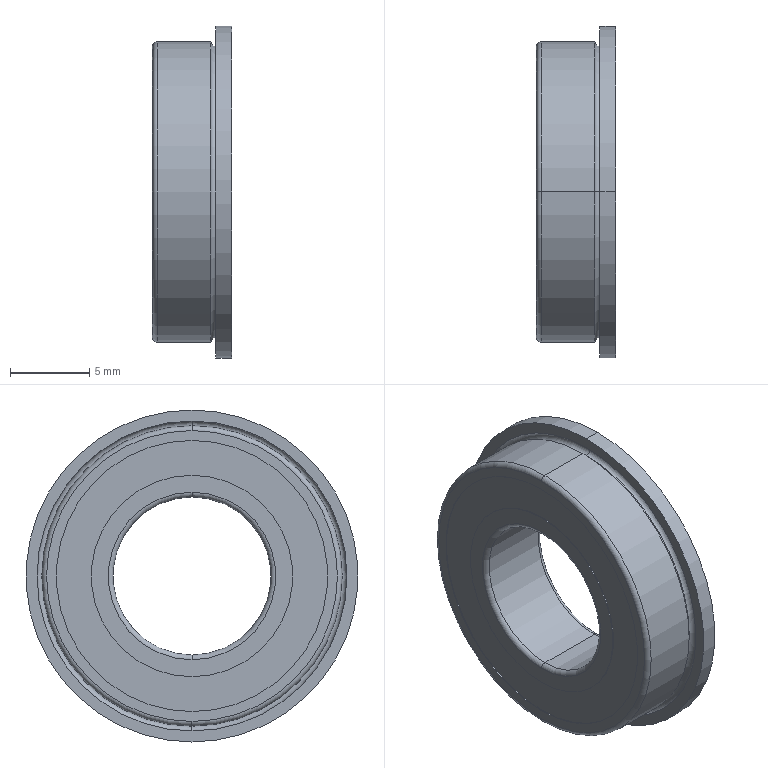Part | STEP file | 11-FL6800ZZ11_FL6800ZZ | 1 solid | 31 faces | box 5 x 21 x 21 mm | volume 1061 mm3 | cylinder 14 | torus 10 | plane 7 | commonest cylinder face diameters 12.74 x4 17.15 x4 10 x2 19 x2 21 x2
STEP:
#1=CARTESIAN_POINT('',(3.7,0.,9.5));
#2=VERTEX_POINT('',#1);
#3=CARTESIAN_POINT('',(4.,0.,9.2));
#4=VERTEX_POINT('',#3);
#5=CARTESIAN_POINT('',(4.,0.,9.5));
#6=DIRECTION('',(0.,-1.,0.));
#7=DIRECTION('',(0.,0.,-1.));
#8=AXIS2_PLACEMENT_3D('',#5,#6,#7);
#9=CIRCLE('',#8,0.3);
#10=EDGE_CURVE('',#2,#4,#9,.T.);
#11=ORIENTED_EDGE('',*,*,#10,.T.);
#12=CARTESIAN_POINT('',(4.,0.,-9.2));
#13=VERTEX_POINT('',#12);
#14=CARTESIAN_POINT('',(4.,0.,0.));
#15=DIRECTION('',(-1.,0.,0.));
#16=DIRECTION('',(0.,0.,1.));
#17=AXIS2_PLACEMENT_3D('',#14,#15,#16);
#18=CIRCLE('',#17,9.2);
#19=EDGE_CURVE('',#4,#13,#18,.T.);
#20=ORIENTED_EDGE('',*,*,#19,.T.);
#21=CARTESIAN_POINT('',(3.7,0.,-9.5));
#22=VERTEX_POINT('',#21);
#23=CARTESIAN_POINT('',(4.,0.,-9.5));
#24=DIRECTION('',(0.,1.,0.));
#25=DIRECTION('',(0.,0.,1.));
#26=AXIS2_PLACEMENT_3D('',#23,#24,#25);
#27=CIRCLE('',#26,0.3);
#28=EDGE_CURVE('',#22,#13,#27,.T.);
#29=ORIENTED_EDGE('',*,*,#28,.F.);
#30=CARTESIAN_POINT('',(3.7,0.,0.));
#31=DIRECTION('',(-1.,0.,0.));
#32=DIRECTION('',(0.,0.,1.));
#33=AXIS2_PLACEMENT_3D('',#30,#31,#32);
#34=CIRCLE('',#33,9.5);
#35=EDGE_CURVE('',#2,#22,#34,.T.);
#36=ORIENTED_EDGE('',*,*,#35,.F.);
#37=EDGE_LOOP('',(#11,#20,#29,#36));
#38=FACE_OUTER_BOUND('',#37,.T.);
#39=CARTESIAN_POINT('',(4.,0.,0.));
#40=DIRECTION('',(-1.,0.,0.));
#41=DIRECTION('',(0.,0.,1.));
#42=AXIS2_PLACEMENT_3D('',#39,#40,#41);
#43=TOROIDAL_SURFACE('',#42,9.5,0.3);
#44=ADVANCED_FACE('',(#38),#43,.F.);
#45=ORIENTED_EDGE('',*,*,#28,.T.);
#46=CARTESIAN_POINT('',(4.,0.,0.));
#47=DIRECTION('',(-1.,0.,0.));
#48=DIRECTION('',(0.,0.,1.));
#49=AXIS2_PLACEMENT_3D('',#46,#47,#48);
#50=CIRCLE('',#49,9.2);
#51=EDGE_CURVE('',#13,#4,#50,.T.);
#52=ORIENTED_EDGE('',*,*,#51,.T.);
#53=ORIENTED_EDGE('',*,*,#10,.F.);
#54=CARTESIAN_POINT('',(3.7,0.,0.));
#55=DIRECTION('',(-1.,0.,0.));
#56=DIRECTION('',(0.,0.,1.));
#57=AXIS2_PLACEMENT_3D('',#54,#55,#56);
#58=CIRCLE('',#57,9.5);
#59=EDGE_CURVE('',#22,#2,#58,.T.);
#60=ORIENTED_EDGE('',*,*,#59,.F.);
#61=EDGE_LOOP('',(#45,#52,#53,#60));
#62=FACE_OUTER_BOUND('',#61,.T.);
#63=CARTESIAN_POINT('',(4.,0.,0.));
#64=DIRECTION('',(-1.,0.,0.));
#65=DIRECTION('',(0.,0.,1.));
#66=AXIS2_PLACEMENT_3D('',#63,#64,#65);
#67=TOROIDAL_SURFACE('',#66,9.5,0.3);
#68=ADVANCED_FACE('',(#62),#67,.F.);
#69=ORIENTED_EDGE('',*,*,#35,.T.);
#70=CARTESIAN_POINT('',(0.3,0.,-9.5));
#71=VERTEX_POINT('',#70);
#72=CARTESIAN_POINT('',(19.,0.,-9.5));
#73=DIRECTION('',(-1.,0.,0.));
#74=VECTOR('',#73,1000.);
#75=LINE('',#72,#74);
#76=EDGE_CURVE('',#22,#71,#75,.T.);
#77=ORIENTED_EDGE('',*,*,#76,.T.);
#78=CARTESIAN_POINT('',(0.3,0.,9.5));
#79=VERTEX_POINT('',#78);
#80=CARTESIAN_POINT('',(0.3,0.,0.));
#81=DIRECTION('',(-1.,0.,0.));
#82=DIRECTION('',(0.,0.,1.));
#83=AXIS2_PLACEMENT_3D('',#80,#81,#82);
#84=CIRCLE('',#83,9.5);
#85=EDGE_CURVE('',#79,#71,#84,.T.);
#86=ORIENTED_EDGE('',*,*,#85,.F.);
#87=CARTESIAN_POINT('',(19.,0.,9.5));
#88=DIRECTION('',(-1.,0.,0.));
#89=VECTOR('',#88,1000.);
#90=LINE('',#87,#89);
#91=EDGE_CURVE('',#2,#79,#90,.T.);
#92=ORIENTED_EDGE('',*,*,#91,.F.);
#93=EDGE_LOOP('',(#69,#77,#86,#92));
#94=FACE_OUTER_BOUND('',#93,.T.);
#95=CARTESIAN_POINT('',(19.,0.,0.));
#96=DIRECTION('',(-1.,0.,0.));
#97=DIRECTION('',(0.,0.,1.));
#98=AXIS2_PLACEMENT_3D('',#95,#96,#97);
#99=CYLINDRICAL_SURFACE('',#98,9.5);
#100=ADVANCED_FACE('',(#94),#99,.T.);
#101=ORIENTED_EDGE('',*,*,#51,.F.);
#102=CARTESIAN_POINT('',(4.,0.,-9.8));
#103=VERTEX_POINT('',#102);
#104=CARTESIAN_POINT('',(4.,0.,-9.5));
#105=DIRECTION('',(0.,1.,0.));
#106=DIRECTION('',(0.,0.,1.));
#107=AXIS2_PLACEMENT_3D('',#104,#105,#106);
#108=CIRCLE('',#107,0.3);
#109=EDGE_CURVE('',#13,#103,#108,.T.);
#110=ORIENTED_EDGE('',*,*,#109,.T.);
#111=CARTESIAN_POINT('',(4.,0.,9.8));
#112=VERTEX_POINT('',#111);
#113=CARTESIAN_POINT('',(4.,0.,0.));
#114=DIRECTION('',(-1.,0.,0.));
#115=DIRECTION('',(0.,0.,1.));
#116=AXIS2_PLACEMENT_3D('',#113,#114,#115);
#117=CIRCLE('',#116,9.8);
#118=EDGE_CURVE('',#103,#112,#117,.T.);
#119=ORIENTED_EDGE('',*,*,#118,.T.);
#120=CARTESIAN_POINT('',(4.,0.,9.5));
#121=DIRECTION('',(0.,-1.,0.));
#122=DIRECTION('',(0.,0.,-1.));
#123=AXIS2_PLACEMENT_3D('',#120,#121,#122);
#124=CIRCLE('',#123,0.3);
#125=EDGE_CURVE('',#4,#112,#124,.T.);
#126=ORIENTED_EDGE('',*,*,#125,.F.);
#127=EDGE_LOOP('',(#101,#110,#119,#126));
#128=FACE_OUTER_BOUND('',#127,.T.);
#129=CARTESIAN_POINT('',(4.,0.,0.));
#130=DIRECTION('',(-1.,0.,0.));
#131=DIRECTION('',(0.,0.,1.));
#132=AXIS2_PLACEMENT_3D('',#129,#130,#131);
#133=TOROIDAL_SURFACE('',#132,9.5,0.3);
#134=ADVANCED_FACE('',(#128),#133,.F.);
#135=CARTESIAN_POINT('',(5.,0.,10.5));
#136=VERTEX_POINT('',#135);
#137=CARTESIAN_POINT('',(5.,0.,-10.5));
#138=VERTEX_POINT('',#137);
#139=CARTESIAN_POINT('',(5.,0.,0.));
#140=DIRECTION('',(-1.,0.,0.));
#141=DIRECTION('',(0.,0.,1.));
#142=AXIS2_PLACEMENT_3D('',#139,#140,#141);
#143=CIRCLE('',#142,10.5);
#144=EDGE_CURVE('',#136,#138,#143,.T.);
#145=ORIENTED_EDGE('',*,*,#144,.T.);
#146=CARTESIAN_POINT('',(4.,0.,-10.5));
#147=VERTEX_POINT('',#146);
#148=CARTESIAN_POINT('',(19.,0.,-10.5));
#149=DIRECTION('',(-1.,0.,0.));
#150=VECTOR('',#149,1000.);
#151=LINE('',#148,#150);
#152=EDGE_CURVE('',#138,#147,#151,.T.);
#153=ORIENTED_EDGE('',*,*,#152,.T.);
#154=CARTESIAN_POINT('',(4.,0.,10.5));
#155=VERTEX_POINT('',#154);
#156=CARTESIAN_POINT('',(4.,0.,0.));
#157=DIRECTION('',(-1.,0.,0.));
#158=DIRECTION('',(0.,0.,1.));
#159=AXIS2_PLACEMENT_3D('',#156,#157,#158);
#160=CIRCLE('',#159,10.5);
#161=EDGE_CURVE('',#155,#147,#160,.T.);
#162=ORIENTED_EDGE('',*,*,#161,.F.);
#163=CARTESIAN_POINT('',(19.,0.,10.5));
#164=DIRECTION('',(-1.,0.,0.));
#165=VECTOR('',#164,1000.);
#166=LINE('',#163,#165);
#167=EDGE_CURVE('',#136,#155,#166,.T.);
#168=ORIENTED_EDGE('',*,*,#167,.F.);
#169=EDGE_LOOP('',(#145,#153,#162,#168));
#170=FACE_OUTER_BOUND('',#169,.T.);
#171=CARTESIAN_POINT('',(19.,0.,0.));
#172=DIRECTION('',(-1.,0.,0.));
#173=DIRECTION('',(0.,0.,1.));
#174=AXIS2_PLACEMENT_3D('',#171,#172,#173);
#175=CYLINDRICAL_SURFACE('',#174,10.5);
#176=ADVANCED_FACE('',(#170),#175,.T.);
#177=CARTESIAN_POINT('',(5.,0.,-8.575));
#178=VERTEX_POINT('',#177);
#179=CARTESIAN_POINT('',(5.,0.,8.575));
#180=VERTEX_POINT('',#179);
#181=CARTESIAN_POINT('',(5.,0.,0.));
#182=DIRECTION('',(-1.,0.,0.));
#183=DIRECTION('',(0.,0.,1.));
#184=AXIS2_PLACEMENT_3D('',#181,#182,#183);
#185=CIRCLE('',#184,8.575);
#186=EDGE_CURVE('',#178,#180,#185,.T.);
#187=ORIENTED_EDGE('',*,*,#186,.F.);
#188=CARTESIAN_POINT('',(4.942,0.,-8.575));
#189=VERTEX_POINT('',#188);
#190=CARTESIAN_POINT('',(19.,0.,-8.575));
#191=DIRECTION('',(-1.,0.,0.));
#192=VECTOR('',#191,1000.);
#193=LINE('',#190,#192);
#194=EDGE_CURVE('',#178,#189,#193,.T.);
#195=ORIENTED_EDGE('',*,*,#194,.T.);
#196=CARTESIAN_POINT('',(4.942,0.,8.575));
#197=VERTEX_POINT('',#196);
#198=CARTESIAN_POINT('',(4.942,0.,0.));
#199=DIRECTION('',(-1.,0.,0.));
#200=DIRECTION('',(0.,0.,1.));
#201=AXIS2_PLACEMENT_3D('',#198,#199,#200);
#202=CIRCLE('',#201,8.575);
#203=EDGE_CURVE('',#189,#197,#202,.T.);
#204=ORIENTED_EDGE('',*,*,#203,.T.);
#205=CARTESIAN_POINT('',(19.,0.,8.575));
#206=DIRECTION('',(-1.,0.,0.));
#207=VECTOR('',#206,1000.);
#208=LINE('',#205,#207);
#209=EDGE_CURVE('',#180,#197,#208,.T.);
#210=ORIENTED_EDGE('',*,*,#209,.F.);
#211=EDGE_LOOP('',(#187,#195,#204,#210));
#212=FACE_OUTER_BOUND('',#211,.T.);
#213=CARTESIAN_POINT('',(19.,0.,0.));
#214=DIRECTION('',(-1.,0.,0.));
#215=DIRECTION('',(0.,0.,1.));
#216=AXIS2_PLACEMENT_3D('',#213,#214,#215);
#217=CYLINDRICAL_SURFACE('',#216,8.575);
#218=ADVANCED_FACE('',(#212),#217,.F.);
#219=CARTESIAN_POINT('',(5.,0.,6.37));
#220=VERTEX_POINT('',#219);
#221=CARTESIAN_POINT('',(5.,0.,-6.37));
#222=VERTEX_POINT('',#221);
#223=CARTESIAN_POINT('',(5.,0.,0.));
#224=DIRECTION('',(-1.,0.,0.));
#225=DIRECTION('',(0.,0.,1.));
#226=AXIS2_PLACEMENT_3D('',#223,#224,#225);
#227=CIRCLE('',#226,6.37);
#228=EDGE_CURVE('',#220,#222,#227,.T.);
#229=ORIENTED_EDGE('',*,*,#228,.T.);
#230=CARTESIAN_POINT('',(4.942,0.,-6.37));
#231=VERTEX_POINT('',#230);
#232=CARTESIAN_POINT('',(19.,0.,-6.37));
#233=DIRECTION('',(-1.,0.,0.));
#234=VECTOR('',#233,1000.);
#235=LINE('',#232,#234);
#236=EDGE_CURVE('',#222,#231,#235,.T.);
#237=ORIENTED_EDGE('',*,*,#236,.T.);
#238=CARTESIAN_POINT('',(4.942,0.,6.37));
#239=VERTEX_POINT('',#238);
#240=CARTESIAN_POINT('',(4.942,0.,0.));
#241=DIRECTION('',(-1.,0.,0.));
#242=DIRECTION('',(0.,0.,1.));
#243=AXIS2_PLACEMENT_3D('',#240,#241,#242);
#244=CIRCLE('',#243,6.37);
#245=EDGE_CURVE('',#239,#231,#244,.T.);
#246=ORIENTED_EDGE('',*,*,#245,.F.);
#247=CARTESIAN_POINT('',(19.,0.,6.37));
#248=DIRECTION('',(-1.,0.,0.));
#249=VECTOR('',#248,1000.);
#250=LINE('',#247,#249);
#251=EDGE_CURVE('',#220,#239,#250,.T.);
#252=ORIENTED_EDGE('',*,*,#251,.F.);
#253=EDGE_LOOP('',(#229,#237,#246,#252));
#254=FACE_OUTER_BOUND('',#253,.T.);
#255=CARTESIAN_POINT('',(19.,0.,0.));
#256=DIRECTION('',(-1.,0.,0.));
#257=DIRECTION('',(0.,0.,1.));
#258=AXIS2_PLACEMENT_3D('',#255,#256,#257);
#259=CYLINDRICAL_SURFACE('',#258,6.37);
#260=ADVANCED_FACE('',(#254),#259,.T.);
#261=CARTESIAN_POINT('',(4.7,0.,5.));
#262=VERTEX_POINT('',#261);
#263=CARTESIAN_POINT('',(4.7,0.,-5.));
#264=VERTEX_POINT('',#263);
#265=CARTESIAN_POINT('',(4.7,0.,0.));
#266=DIRECTION('',(-1.,0.,0.));
#267=DIRECTION('',(0.,0.,1.));
#268=AXIS2_PLACEMENT_3D('',#265,#266,#267);
#269=CIRCLE('',#268,5.);
#270=EDGE_CURVE('',#262,#264,#269,.T.);
#271=ORIENTED_EDGE('',*,*,#270,.T.);
#272=CARTESIAN_POINT('',(5.,0.,-5.3));
#273=VERTEX_POINT('',#272);
#274=CARTESIAN_POINT('',(4.7,0.,-5.3));
#275=DIRECTION('',(0.,1.,0.));
#276=DIRECTION('',(0.,0.,1.));
#277=AXIS2_PLACEMENT_3D('',#274,#275,#276);
#278=CIRCLE('',#277,0.3);
#279=EDGE_CURVE('',#264,#273,#278,.T.);
#280=ORIENTED_EDGE('',*,*,#279,.T.);
#281=CARTESIAN_POINT('',(5.,0.,5.3));
#282=VERTEX_POINT('',#281);
#283=CARTESIAN_POINT('',(5.,0.,0.));
#284=DIRECTION('',(-1.,0.,0.));
#285=DIRECTION('',(0.,0.,1.));
#286=AXIS2_PLACEMENT_3D('',#283,#284,#285);
#287=CIRCLE('',#286,5.3);
#288=EDGE_CURVE('',#282,#273,#287,.T.);
#289=ORIENTED_EDGE('',*,*,#288,.F.);
#290=CARTESIAN_POINT('',(4.7,0.,5.3));
#291=DIRECTION('',(0.,-1.,0.));
#292=DIRECTION('',(0.,0.,-1.));
#293=AXIS2_PLACEMENT_3D('',#290,#291,#292);
#294=CIRCLE('',#293,0.3);
#295=EDGE_CURVE('',#262,#282,#294,.T.);
#296=ORIENTED_EDGE('',*,*,#295,.F.);
#297=EDGE_LOOP('',(#271,#280,#289,#296));
#298=FACE_OUTER_BOUND('',#297,.T.);
#299=CARTESIAN_POINT('',(4.7,0.,0.));
#300=DIRECTION('',(-1.,0.,0.));
#301=DIRECTION('',(0.,0.,1.));
#302=AXIS2_PLACEMENT_3D('',#299,#300,#301);
#303=TOROIDAL_SURFACE('',#302,5.3,0.3);
#304=ADVANCED_FACE('',(#298),#303,.T.);
#305=CARTESIAN_POINT('',(4.7,0.,0.));
#306=DIRECTION('',(-1.,0.,0.));
#307=DIRECTION('',(0.,0.,1.));
#308=AXIS2_PLACEMENT_3D('',#305,#306,#307);
#309=CIRCLE('',#308,5.);
#310=EDGE_CURVE('',#264,#262,#309,.T.);
#311=ORIENTED_EDGE('',*,*,#310,.F.);
#312=CARTESIAN_POINT('',(0.3,0.,-5.));
#313=VERTEX_POINT('',#312);
#314=CARTESIAN_POINT('',(19.,0.,-5.));
#315=DIRECTION('',(-1.,0.,0.));
#316=VECTOR('',#315,1000.);
#317=LINE('',#314,#316);
#318=EDGE_CURVE('',#264,#313,#317,.T.);
#319=ORIENTED_EDGE('',*,*,#318,.T.);
#320=CARTESIAN_POINT('',(0.3,0.,5.));
#321=VERTEX_POINT('',#320);
#322=CARTESIAN_POINT('',(0.3,0.,0.));
#323=DIRECTION('',(-1.,0.,0.));
#324=DIRECTION('',(0.,0.,1.));
#325=AXIS2_PLACEMENT_3D('',#322,#323,#324);
#326=CIRCLE('',#325,5.);
#327=EDGE_CURVE('',#313,#321,#326,.T.);
#328=ORIENTED_EDGE('',*,*,#327,.T.);
#329=CARTESIAN_POINT('',(19.,0.,5.));
#330=DIRECTION('',(-1.,0.,0.));
#331=VECTOR('',#330,1000.);
#332=LINE('',#329,#331);
#333=EDGE_CURVE('',#262,#321,#332,.T.);
#334=ORIENTED_EDGE('',*,*,#333,.F.);
#335=EDGE_LOOP('',(#311,#319,#328,#334));
#336=FACE_OUTER_BOUND('',#335,.T.);
#337=CARTESIAN_POINT('',(19.,0.,0.));
#338=DIRECTION('',(-1.,0.,0.));
#339=DIRECTION('',(0.,0.,1.));
#340=AXIS2_PLACEMENT_3D('',#337,#338,#339);
#341=CYLINDRICAL_SURFACE('',#340,5.);
#342=ADVANCED_FACE('',(#336),#341,.F.);
#343=CARTESIAN_POINT('',(0.,0.,5.3));
#344=VERTEX_POINT('',#343);
#345=CARTESIAN_POINT('',(0.,0.,-5.3));
#346=VERTEX_POINT('',#345);
#347=CARTESIAN_POINT('',(0.,0.,0.));
#348=DIRECTION('',(-1.,0.,0.));
#349=DIRECTION('',(0.,0.,1.));
#350=AXIS2_PLACEMENT_3D('',#347,#348,#349);
#351=CIRCLE('',#350,5.3);
#352=EDGE_CURVE('',#344,#346,#351,.T.);
#353=ORIENTED_EDGE('',*,*,#352,.T.);
#354=CARTESIAN_POINT('',(0.3,0.,-5.3));
#355=DIRECTION('',(0.,1.,0.));
#356=DIRECTION('',(0.,0.,1.));
#357=AXIS2_PLACEMENT_3D('',#354,#355,#356);
#358=CIRCLE('',#357,0.3);
#359=EDGE_CURVE('',#346,#313,#358,.T.);
#360=ORIENTED_EDGE('',*,*,#359,.T.);
#361=CARTESIAN_POINT('',(0.3,0.,0.));
#362=DIRECTION('',(-1.,0.,0.));
#363=DIRECTION('',(0.,0.,1.));
#364=AXIS2_PLACEMENT_3D('',#361,#362,#363);
#365=CIRCLE('',#364,5.);
#366=EDGE_CURVE('',#321,#313,#365,.T.);
#367=ORIENTED_EDGE('',*,*,#366,.F.);
#368=CARTESIAN_POINT('',(0.3,0.,5.3));
#369=DIRECTION('',(0.,-1.,0.));
#370=DIRECTION('',(0.,0.,-1.));
#371=AXIS2_PLACEMENT_3D('',#368,#369,#370);
#372=CIRCLE('',#371,0.3);
#373=EDGE_CURVE('',#344,#321,#372,.T.);
#374=ORIENTED_EDGE('',*,*,#373,.F.);
#375=EDGE_LOOP('',(#353,#360,#367,#374));
#376=FACE_OUTER_BOUND('',#375,.T.);
#377=CARTESIAN_POINT('',(0.3,0.,0.));
#378=DIRECTION('',(-1.,0.,0.));
#379=DIRECTION('',(0.,0.,1.));
#380=AXIS2_PLACEMENT_3D('',#377,#378,#379);
#381=TOROIDAL_SURFACE('',#380,5.3,0.3);
#382=ADVANCED_FACE('',(#376),#381,.T.);
#383=CARTESIAN_POINT('',(0.0575,0.,6.37));
#384=VERTEX_POINT('',#383);
#385=CARTESIAN_POINT('',(0.0575,0.,-6.37));
#386=VERTEX_POINT('',#385);
#387=CARTESIAN_POINT('',(0.0575,0.,0.));
#388=DIRECTION('',(-1.,0.,0.));
#389=DIRECTION('',(0.,0.,1.));
#390=AXIS2_PLACEMENT_3D('',#387,#388,#389);
#391=CIRCLE('',#390,6.37);
#392=EDGE_CURVE('',#384,#386,#391,.T.);
#393=ORIENTED_EDGE('',*,*,#392,.T.);
#394=CARTESIAN_POINT('',(0.,0.,-6.37));
#395=VERTEX_POINT('',#394);
#396=CARTESIAN_POINT('',(19.,0.,-6.37));
#397=DIRECTION('',(-1.,0.,0.));
#398=VECTOR('',#397,1000.);
#399=LINE('',#396,#398);
#400=EDGE_CURVE('',#386,#395,#399,.T.);
#401=ORIENTED_EDGE('',*,*,#400,.T.);
#402=CARTESIAN_POINT('',(0.,0.,6.37));
#403=VERTEX_POINT('',#402);
#404=CARTESIAN_POINT('',(0.,0.,0.));
#405=DIRECTION('',(-1.,0.,0.));
#406=DIRECTION('',(0.,0.,1.));
#407=AXIS2_PLACEMENT_3D('',#404,#405,#406);
#408=CIRCLE('',#407,6.37);
#409=EDGE_CURVE('',#403,#395,#408,.T.);
#410=ORIENTED_EDGE('',*,*,#409,.F.);
#411=CARTESIAN_POINT('',(19.,0.,6.37));
#412=DIRECTION('',(-1.,0.,0.));
#413=VECTOR('',#412,1000.);
#414=LINE('',#411,#413);
#415=EDGE_CURVE('',#384,#403,#414,.T.);
#416=ORIENTED_EDGE('',*,*,#415,.F.);
#417=EDGE_LOOP('',(#393,#401,#410,#416));
#418=FACE_OUTER_BOUND('',#417,.T.);
#419=CARTESIAN_POINT('',(19.,0.,0.));
#420=DIRECTION('',(-1.,0.,0.));
#421=DIRECTION('',(0.,0.,1.));
#422=AXIS2_PLACEMENT_3D('',#419,#420,#421);
#423=CYLINDRICAL_SURFACE('',#422,6.37);
#424=ADVANCED_FACE('',(#418),#423,.T.);
#425=CARTESIAN_POINT('',(0.0575,0.,-8.575));
#426=VERTEX_POINT('',#425);
#427=CARTESIAN_POINT('',(0.0575,0.,8.575));
#428=VERTEX_POINT('',#427);
#429=CARTESIAN_POINT('',(0.0575,0.,0.));
#430=DIRECTION('',(-1.,0.,0.));
#431=DIRECTION('',(0.,0.,1.));
#432=AXIS2_PLACEMENT_3D('',#429,#430,#431);
#433=CIRCLE('',#432,8.575);
#434=EDGE_CURVE('',#426,#428,#433,.T.);
#435=ORIENTED_EDGE('',*,*,#434,.F.);
#436=CARTESIAN_POINT('',(0.,0.,-8.575));
#437=VERTEX_POINT('',#436);
#438=CARTESIAN_POINT('',(19.,0.,-8.575));
#439=DIRECTION('',(-1.,0.,0.));
#440=VECTOR('',#439,1000.);
#441=LINE('',#438,#440);
#442=EDGE_CURVE('',#426,#437,#441,.T.);
#443=ORIENTED_EDGE('',*,*,#442,.T.);
#444=CARTESIAN_POINT('',(0.,0.,8.575));
#445=VERTEX_POINT('',#444);
#446=CARTESIAN_POINT('',(0.,0.,0.));
#447=DIRECTION('',(-1.,0.,0.));
#448=DIRECTION('',(0.,0.,1.));
#449=AXIS2_PLACEMENT_3D('',#446,#447,#448);
#450=CIRCLE('',#449,8.575);
#451=EDGE_CURVE('',#437,#445,#450,.T.);
#452=ORIENTED_EDGE('',*,*,#451,.T.);
#453=CARTESIAN_POINT('',(19.,0.,8.575));
#454=DIRECTION('',(-1.,0.,0.));
#455=VECTOR('',#454,1000.);
#456=LINE('',#453,#455);
#457=EDGE_CURVE('',#428,#445,#456,.T.);
#458=ORIENTED_EDGE('',*,*,#457,.F.);
#459=EDGE_LOOP('',(#435,#443,#452,#458));
#460=FACE_OUTER_BOUND('',#459,.T.);
#461=CARTESIAN_POINT('',(19.,0.,0.));
#462=DIRECTION('',(-1.,0.,0.));
#463=DIRECTION('',(0.,0.,1.));
#464=AXIS2_PLACEMENT_3D('',#461,#462,#463);
#465=CYLINDRICAL_SURFACE('',#464,8.575);
#466=ADVANCED_FACE('',(#460),#465,.F.);
#467=ORIENTED_EDGE('',*,*,#85,.T.);
#468=CARTESIAN_POINT('',(0.,0.,-9.2));
#469=VERTEX_POINT('',#468);
#470=CARTESIAN_POINT('',(0.3,0.,-9.2));
#471=DIRECTION('',(0.,1.,0.));
#472=DIRECTION('',(0.,0.,1.));
#473=AXIS2_PLACEMENT_3D('',#470,#471,#472);
#474=CIRCLE('',#473,0.3);
#475=EDGE_CURVE('',#71,#469,#474,.T.);
#476=ORIENTED_EDGE('',*,*,#475,.T.);
#477=CARTESIAN_POINT('',(0.,0.,9.2));
#478=VERTEX_POINT('',#477);
#479=CARTESIAN_POINT('',(0.,0.,0.));
#480=DIRECTION('',(-1.,0.,0.));
#481=DIRECTION('',(0.,0.,1.));
#482=AXIS2_PLACEMENT_3D('',#479,#480,#481);
#483=CIRCLE('',#482,9.2);
#484=EDGE_CURVE('',#478,#469,#483,.T.);
#485=ORIENTED_EDGE('',*,*,#484,.F.);
#486=CARTESIAN_POINT('',(0.3,0.,9.2));
#487=DIRECTION('',(0.,-1.,0.));
#488=DIRECTION('',(0.,0.,-1.));
#489=AXIS2_PLACEMENT_3D('',#486,#487,#488);
#490=CIRCLE('',#489,0.3);
#491=EDGE_CURVE('',#79,#478,#490,.T.);
#492=ORIENTED_EDGE('',*,*,#491,.F.);
#493=EDGE_LOOP('',(#467,#476,#485,#492));
#494=FACE_OUTER_BOUND('',#493,.T.);
#495=CARTESIAN_POINT('',(0.3,0.,0.));
#496=DIRECTION('',(-1.,0.,0.));
#497=DIRECTION('',(0.,0.,1.));
#498=AXIS2_PLACEMENT_3D('',#495,#496,#497);
#499=TOROIDAL_SURFACE('',#498,9.2,0.3);
#500=ADVANCED_FACE('',(#494),#499,.T.);
#501=ORIENTED_EDGE('',*,*,#475,.F.);
#502=CARTESIAN_POINT('',(0.3,0.,0.));
#503=DIRECTION('',(-1.,0.,0.));
#504=DIRECTION('',(0.,0.,1.));
#505=AXIS2_PLACEMENT_3D('',#502,#503,#504);
#506=CIRCLE('',#505,9.5);
#507=EDGE_CURVE('',#71,#79,#506,.T.);
#508=ORIENTED_EDGE('',*,*,#507,.T.);
#509=ORIENTED_EDGE('',*,*,#491,.T.);
#510=CARTESIAN_POINT('',(0.,0.,0.));
#511=DIRECTION('',(-1.,0.,0.));
#512=DIRECTION('',(0.,0.,1.));
#513=AXIS2_PLACEMENT_3D('',#510,#511,#512);
#514=CIRCLE('',#513,9.2);
#515=EDGE_CURVE('',#469,#478,#514,.T.);
#516=ORIENTED_EDGE('',*,*,#515,.F.);
#517=EDGE_LOOP('',(#501,#508,#509,#516));
#518=FACE_OUTER_BOUND('',#517,.T.);
#519=CARTESIAN_POINT('',(0.3,0.,0.));
#520=DIRECTION('',(-1.,0.,0.));
#521=DIRECTION('',(0.,0.,1.));
#522=AXIS2_PLACEMENT_3D('',#519,#520,#521);
#523=TOROIDAL_SURFACE('',#522,9.2,0.3);
#524=ADVANCED_FACE('',(#518),#523,.T.);
#525=CARTESIAN_POINT('',(0.,0.,0.));
#526=DIRECTION('',(-1.,0.,0.));
#527=DIRECTION('',(0.,0.,1.));
#528=AXIS2_PLACEMENT_3D('',#525,#526,#527);
#529=CIRCLE('',#528,8.575);
#530=EDGE_CURVE('',#445,#437,#529,.T.);
#531=ORIENTED_EDGE('',*,*,#530,.F.);
#532=ORIENTED_EDGE('',*,*,#451,.F.);
#533=EDGE_LOOP('',(#531,#532));
#534=FACE_BOUND('',#533,.T.);
#535=ORIENTED_EDGE('',*,*,#484,.T.);
#536=ORIENTED_EDGE('',*,*,#515,.T.);
#537=EDGE_LOOP('',(#535,#536));
#538=FACE_OUTER_BOUND('',#537,.T.);
#539=CARTESIAN_POINT('',(0.,9.2,0.));
#540=DIRECTION('',(1.,0.,0.));
#541=DIRECTION('',(0.,0.,-1.));
#542=AXIS2_PLACEMENT_3D('',#539,#540,#541);
#543=PLANE('',#542);
#544=ADVANCED_FACE('',(#534,#538),#543,.F.);
#545=ORIENTED_EDGE('',*,*,#442,.F.);
#546=CARTESIAN_POINT('',(0.0575,0.,0.));
#547=DIRECTION('',(-1.,0.,0.));
#548=DIRECTION('',(0.,0.,1.));
#549=AXIS2_PLACEMENT_3D('',#546,#547,#548);
#550=CIRCLE('',#549,8.575);
#551=EDGE_CURVE('',#428,#426,#550,.T.);
#552=ORIENTED_EDGE('',*,*,#551,.F.);
#553=ORIENTED_EDGE('',*,*,#457,.T.);
#554=ORIENTED_EDGE('',*,*,#530,.T.);
#555=EDGE_LOOP('',(#545,#552,#553,#554));
#556=FACE_OUTER_BOUND('',#555,.T.);
#557=CARTESIAN_POINT('',(19.,0.,0.));
#558=DIRECTION('',(-1.,0.,0.));
#559=DIRECTION('',(0.,0.,1.));
#560=AXIS2_PLACEMENT_3D('',#557,#558,#559);
#561=CYLINDRICAL_SURFACE('',#560,8.575);
#562=ADVANCED_FACE('',(#556),#561,.F.);
#563=ORIENTED_EDGE('',*,*,#392,.F.);
#564=CARTESIAN_POINT('',(0.0575,0.,0.));
#565=DIRECTION('',(-1.,0.,0.));
#566=DIRECTION('',(0.,0.,1.));
#567=AXIS2_PLACEMENT_3D('',#564,#565,#566);
#568=CIRCLE('',#567,6.37);
#569=EDGE_CURVE('',#386,#384,#568,.T.);
#570=ORIENTED_EDGE('',*,*,#569,.F.);
#571=EDGE_LOOP('',(#563,#570));
#572=FACE_BOUND('',#571,.T.);
#573=ORIENTED_EDGE('',*,*,#551,.T.);
#574=ORIENTED_EDGE('',*,*,#434,.T.);
#575=EDGE_LOOP('',(#573,#574));
#576=FACE_OUTER_BOUND('',#575,.T.);
#577=CARTESIAN_POINT('',(0.0575,8.575,0.));
#578=DIRECTION('',(1.,0.,0.));
#579=DIRECTION('',(0.,0.,-1.));
#580=AXIS2_PLACEMENT_3D('',#577,#578,#579);
#581=PLANE('',#580);
#582=ADVANCED_FACE('',(#572,#576),#581,.F.);
#583=ORIENTED_EDGE('',*,*,#400,.F.);
#584=ORIENTED_EDGE('',*,*,#569,.T.);
#585=ORIENTED_EDGE('',*,*,#415,.T.);
#586=CARTESIAN_POINT('',(0.,0.,0.));
#587=DIRECTION('',(-1.,0.,0.));
#588=DIRECTION('',(0.,0.,1.));
#589=AXIS2_PLACEMENT_3D('',#586,#587,#588);
#590=CIRCLE('',#589,6.37);
#591=EDGE_CURVE('',#395,#403,#590,.T.);
#592=ORIENTED_EDGE('',*,*,#591,.F.);
#593=EDGE_LOOP('',(#583,#584,#585,#592));
#594=FACE_OUTER_BOUND('',#593,.T.);
#595=CARTESIAN_POINT('',(19.,0.,0.));
#596=DIRECTION('',(-1.,0.,0.));
#597=DIRECTION('',(0.,0.,1.));
#598=AXIS2_PLACEMENT_3D('',#595,#596,#597);
#599=CYLINDRICAL_SURFACE('',#598,6.37);
#600=ADVANCED_FACE('',(#594),#599,.T.);
#601=ORIENTED_EDGE('',*,*,#352,.F.);
#602=CARTESIAN_POINT('',(0.,0.,0.));
#603=DIRECTION('',(-1.,0.,0.));
#604=DIRECTION('',(0.,0.,1.));
#605=AXIS2_PLACEMENT_3D('',#602,#603,#604);
#606=CIRCLE('',#605,5.3);
#607=EDGE_CURVE('',#346,#344,#606,.T.);
#608=ORIENTED_EDGE('',*,*,#607,.F.);
#609=EDGE_LOOP('',(#601,#608));
#610=FACE_BOUND('',#609,.T.);
#611=ORIENTED_EDGE('',*,*,#409,.T.);
#612=ORIENTED_EDGE('',*,*,#591,.T.);
#613=EDGE_LOOP('',(#611,#612));
#614=FACE_OUTER_BOUND('',#613,.T.);
#615=CARTESIAN_POINT('',(0.,6.37,0.));
#616=DIRECTION('',(1.,0.,0.));
#617=DIRECTION('',(0.,0.,-1.));
#618=AXIS2_PLACEMENT_3D('',#615,#616,#617);
#619=PLANE('',#618);
#620=ADVANCED_FACE('',(#610,#614),#619,.F.);
#621=ORIENTED_EDGE('',*,*,#359,.F.);
#622=ORIENTED_EDGE('',*,*,#607,.T.);
#623=ORIENTED_EDGE('',*,*,#373,.T.);
#624=ORIENTED_EDGE('',*,*,#327,.F.);
#625=EDGE_LOOP('',(#621,#622,#623,#624));
#626=FACE_OUTER_BOUND('',#625,.T.);
#627=CARTESIAN_POINT('',(0.3,0.,0.));
#628=DIRECTION('',(-1.,0.,0.));
#629=DIRECTION('',(0.,0.,1.));
#630=AXIS2_PLACEMENT_3D('',#627,#628,#629);
#631=TOROIDAL_SURFACE('',#630,5.3,0.3);
#632=ADVANCED_FACE('',(#626),#631,.T.);
#633=ORIENTED_EDGE('',*,*,#318,.F.);
#634=ORIENTED_EDGE('',*,*,#270,.F.);
#635=ORIENTED_EDGE('',*,*,#333,.T.);
#636=ORIENTED_EDGE('',*,*,#366,.T.);
#637=EDGE_LOOP('',(#633,#634,#635,#636));
#638=FACE_OUTER_BOUND('',#637,.T.);
#639=CARTESIAN_POINT('',(19.,0.,0.));
#640=DIRECTION('',(-1.,0.,0.));
#641=DIRECTION('',(0.,0.,1.));
#642=AXIS2_PLACEMENT_3D('',#639,#640,#641);
#643=CYLINDRICAL_SURFACE('',#642,5.);
#644=ADVANCED_FACE('',(#638),#643,.F.);
#645=ORIENTED_EDGE('',*,*,#279,.F.);
#646=ORIENTED_EDGE('',*,*,#310,.T.);
#647=ORIENTED_EDGE('',*,*,#295,.T.);
#648=CARTESIAN_POINT('',(5.,0.,0.));
#649=DIRECTION('',(-1.,0.,0.));
#650=DIRECTION('',(0.,0.,1.));
#651=AXIS2_PLACEMENT_3D('',#648,#649,#650);
#652=CIRCLE('',#651,5.3);
#653=EDGE_CURVE('',#273,#282,#652,.T.);
#654=ORIENTED_EDGE('',*,*,#653,.F.);
#655=EDGE_LOOP('',(#645,#646,#647,#654));
#656=FACE_OUTER_BOUND('',#655,.T.);
#657=CARTESIAN_POINT('',(4.7,0.,0.));
#658=DIRECTION('',(-1.,0.,0.));
#659=DIRECTION('',(0.,0.,1.));
#660=AXIS2_PLACEMENT_3D('',#657,#658,#659);
#661=TOROIDAL_SURFACE('',#660,5.3,0.3);
#662=ADVANCED_FACE('',(#656),#661,.T.);
#663=ORIENTED_EDGE('',*,*,#228,.F.);
#664=CARTESIAN_POINT('',(5.,0.,0.));
#665=DIRECTION('',(-1.,0.,0.));
#666=DIRECTION('',(0.,0.,1.));
#667=AXIS2_PLACEMENT_3D('',#664,#665,#666);
#668=CIRCLE('',#667,6.37);
#669=EDGE_CURVE('',#222,#220,#668,.T.);
#670=ORIENTED_EDGE('',*,*,#669,.F.);
#671=EDGE_LOOP('',(#663,#670));
#672=FACE_OUTER_BOUND('',#671,.T.);
#673=ORIENTED_EDGE('',*,*,#288,.T.);
#674=ORIENTED_EDGE('',*,*,#653,.T.);
#675=EDGE_LOOP('',(#673,#674));
#676=FACE_BOUND('',#675,.T.);
#677=CARTESIAN_POINT('',(5.,5.3,0.));
#678=DIRECTION('',(-1.,0.,0.));
#679=DIRECTION('',(0.,0.,1.));
#680=AXIS2_PLACEMENT_3D('',#677,#678,#679);
#681=PLANE('',#680);
#682=ADVANCED_FACE('',(#672,#676),#681,.F.);
#683=ORIENTED_EDGE('',*,*,#236,.F.);
#684=ORIENTED_EDGE('',*,*,#669,.T.);
#685=ORIENTED_EDGE('',*,*,#251,.T.);
#686=CARTESIAN_POINT('',(4.942,0.,0.));
#687=DIRECTION('',(-1.,0.,0.));
#688=DIRECTION('',(0.,0.,1.));
#689=AXIS2_PLACEMENT_3D('',#686,#687,#688);
#690=CIRCLE('',#689,6.37);
#691=EDGE_CURVE('',#231,#239,#690,.T.);
#692=ORIENTED_EDGE('',*,*,#691,.F.);
#693=EDGE_LOOP('',(#683,#684,#685,#692));
#694=FACE_OUTER_BOUND('',#693,.T.);
#695=CARTESIAN_POINT('',(19.,0.,0.));
#696=DIRECTION('',(-1.,0.,0.));
#697=DIRECTION('',(0.,0.,1.));
#698=AXIS2_PLACEMENT_3D('',#695,#696,#697);
#699=CYLINDRICAL_SURFACE('',#698,6.37);
#700=ADVANCED_FACE('',(#694),#699,.T.);
#701=CARTESIAN_POINT('',(4.942,0.,0.));
#702=DIRECTION('',(-1.,0.,0.));
#703=DIRECTION('',(0.,0.,1.));
#704=AXIS2_PLACEMENT_3D('',#701,#702,#703);
#705=CIRCLE('',#704,8.575);
#706=EDGE_CURVE('',#197,#189,#705,.T.);
#707=ORIENTED_EDGE('',*,*,#706,.F.);
#708=ORIENTED_EDGE('',*,*,#203,.F.);
#709=EDGE_LOOP('',(#707,#708));
#710=FACE_OUTER_BOUND('',#709,.T.);
#711=ORIENTED_EDGE('',*,*,#245,.T.);
#712=ORIENTED_EDGE('',*,*,#691,.T.);
#713=EDGE_LOOP('',(#711,#712));
#714=FACE_BOUND('',#713,.T.);
#715=CARTESIAN_POINT('',(4.942,6.37,0.));
#716=DIRECTION('',(-1.,0.,0.));
#717=DIRECTION('',(0.,0.,1.));
#718=AXIS2_PLACEMENT_3D('',#715,#716,#717);
#719=PLANE('',#718);
#720=ADVANCED_FACE('',(#710,#714),#719,.F.);
#721=ORIENTED_EDGE('',*,*,#194,.F.);
#722=CARTESIAN_POINT('',(5.,0.,0.));
#723=DIRECTION('',(-1.,0.,0.));
#724=DIRECTION('',(0.,0.,1.));
#725=AXIS2_PLACEMENT_3D('',#722,#723,#724);
#726=CIRCLE('',#725,8.575);
#727=EDGE_CURVE('',#180,#178,#726,.T.);
#728=ORIENTED_EDGE('',*,*,#727,.F.);
#729=ORIENTED_EDGE('',*,*,#209,.T.);
#730=ORIENTED_EDGE('',*,*,#706,.T.);
#731=EDGE_LOOP('',(#721,#728,#729,#730));
#732=FACE_OUTER_BOUND('',#731,.T.);
#733=CARTESIAN_POINT('',(19.,0.,0.));
#734=DIRECTION('',(-1.,0.,0.));
#735=DIRECTION('',(0.,0.,1.));
#736=AXIS2_PLACEMENT_3D('',#733,#734,#735);
#737=CYLINDRICAL_SURFACE('',#736,8.575);
#738=ADVANCED_FACE('',(#732),#737,.F.);
#739=ORIENTED_EDGE('',*,*,#144,.F.);
#740=CARTESIAN_POINT('',(5.,0.,0.));
#741=DIRECTION('',(-1.,0.,0.));
#742=DIRECTION('',(0.,0.,1.));
#743=AXIS2_PLACEMENT_3D('',#740,#741,#742);
#744=CIRCLE('',#743,10.5);
#745=EDGE_CURVE('',#138,#136,#744,.T.);
#746=ORIENTED_EDGE('',*,*,#745,.F.);
#747=EDGE_LOOP('',(#739,#746));
#748=FACE_OUTER_BOUND('',#747,.T.);
#749=ORIENTED_EDGE('',*,*,#727,.T.);
#750=ORIENTED_EDGE('',*,*,#186,.T.);
#751=EDGE_LOOP('',(#749,#750));
#752=FACE_BOUND('',#751,.T.);
#753=CARTESIAN_POINT('',(5.,8.575,0.));
#754=DIRECTION('',(-1.,0.,0.));
#755=DIRECTION('',(0.,0.,1.));
#756=AXIS2_PLACEMENT_3D('',#753,#754,#755);
#757=PLANE('',#756);
#758=ADVANCED_FACE('',(#748,#752),#757,.F.);
#759=ORIENTED_EDGE('',*,*,#152,.F.);
#760=ORIENTED_EDGE('',*,*,#745,.T.);
#761=ORIENTED_EDGE('',*,*,#167,.T.);
#762=CARTESIAN_POINT('',(4.,0.,0.));
#763=DIRECTION('',(-1.,0.,0.));
#764=DIRECTION('',(0.,0.,1.));
#765=AXIS2_PLACEMENT_3D('',#762,#763,#764);
#766=CIRCLE('',#765,10.5);
#767=EDGE_CURVE('',#147,#155,#766,.T.);
#768=ORIENTED_EDGE('',*,*,#767,.F.);
#769=EDGE_LOOP('',(#759,#760,#761,#768));
#770=FACE_OUTER_BOUND('',#769,.T.);
#771=CARTESIAN_POINT('',(19.,0.,0.));
#772=DIRECTION('',(-1.,0.,0.));
#773=DIRECTION('',(0.,0.,1.));
#774=AXIS2_PLACEMENT_3D('',#771,#772,#773);
#775=CYLINDRICAL_SURFACE('',#774,10.5);
#776=ADVANCED_FACE('',(#770),#775,.T.);
#777=CARTESIAN_POINT('',(4.,0.,0.));
#778=DIRECTION('',(-1.,0.,0.));
#779=DIRECTION('',(0.,0.,1.));
#780=AXIS2_PLACEMENT_3D('',#777,#778,#779);
#781=CIRCLE('',#780,9.8);
#782=EDGE_CURVE('',#112,#103,#781,.T.);
#783=ORIENTED_EDGE('',*,*,#782,.F.);
#784=ORIENTED_EDGE('',*,*,#118,.F.);
#785=EDGE_LOOP('',(#783,#784));
#786=FACE_BOUND('',#785,.T.);
#787=ORIENTED_EDGE('',*,*,#161,.T.);
#788=ORIENTED_EDGE('',*,*,#767,.T.);
#789=EDGE_LOOP('',(#787,#788));
#790=FACE_OUTER_BOUND('',#789,.T.);
#791=CARTESIAN_POINT('',(4.,10.5,0.));
#792=DIRECTION('',(1.,0.,0.));
#793=DIRECTION('',(0.,0.,-1.));
#794=AXIS2_PLACEMENT_3D('',#791,#792,#793);
#795=PLANE('',#794);
#796=ADVANCED_FACE('',(#786,#790),#795,.F.);
#797=ORIENTED_EDGE('',*,*,#19,.F.);
#798=ORIENTED_EDGE('',*,*,#125,.T.);
#799=ORIENTED_EDGE('',*,*,#782,.T.);
#800=ORIENTED_EDGE('',*,*,#109,.F.);
#801=EDGE_LOOP('',(#797,#798,#799,#800));
#802=FACE_OUTER_BOUND('',#801,.T.);
#803=CARTESIAN_POINT('',(4.,0.,0.));
#804=DIRECTION('',(-1.,0.,0.));
#805=DIRECTION('',(0.,0.,1.));
#806=AXIS2_PLACEMENT_3D('',#803,#804,#805);
#807=TOROIDAL_SURFACE('',#806,9.5,0.3);
#808=ADVANCED_FACE('',(#802),#807,.F.);
#809=ORIENTED_EDGE('',*,*,#76,.F.);
#810=ORIENTED_EDGE('',*,*,#59,.T.);
#811=ORIENTED_EDGE('',*,*,#91,.T.);
#812=ORIENTED_EDGE('',*,*,#507,.F.);
#813=EDGE_LOOP('',(#809,#810,#811,#812));
#814=FACE_OUTER_BOUND('',#813,.T.);
#815=CARTESIAN_POINT('',(19.,0.,0.));
#816=DIRECTION('',(-1.,0.,0.));
#817=DIRECTION('',(0.,0.,1.));
#818=AXIS2_PLACEMENT_3D('',#815,#816,#817);
#819=CYLINDRICAL_SURFACE('',#818,9.5);
#820=ADVANCED_FACE('',(#814),#819,.T.);
#821=CLOSED_SHELL('',(#44,#68,#100,#134,#176,#218,#260,#304,#342,#382,#424,#466,#500,#524,#544,#562,#582,#600,#620,#632,#644,#662,#682,#700,#720,#738,#758,#776,#796,#808,#820));
#822=MANIFOLD_SOLID_BREP('',#821);
#823=CARTESIAN_POINT('',(0.,0.,0.));
#824=DIRECTION('',(0.,0.,1.));
#825=DIRECTION('',(1.,0.,0.));
#826=AXIS2_PLACEMENT_3D('',#823,#824,#825);
#827=(LENGTH_UNIT()NAMED_UNIT(*)SI_UNIT(.MILLI.,.METRE.));
#828=UNCERTAINTY_MEASURE_WITH_UNIT(LENGTH_MEASURE(0.00001),#827,'','');
#829=(NAMED_UNIT(*)PLANE_ANGLE_UNIT()SI_UNIT($,.RADIAN.));
#830=(NAMED_UNIT(*)SI_UNIT($,.STERADIAN.)SOLID_ANGLE_UNIT());
#831=(GEOMETRIC_REPRESENTATION_CONTEXT(3)GLOBAL_UNCERTAINTY_ASSIGNED_CONTEXT((#828))GLOBAL_UNIT_ASSIGNED_CONTEXT((#827,#829,#830))REPRESENTATION_CONTEXT('',''));
#832=ADVANCED_BREP_SHAPE_REPRESENTATION('',(#822,#826),#831);